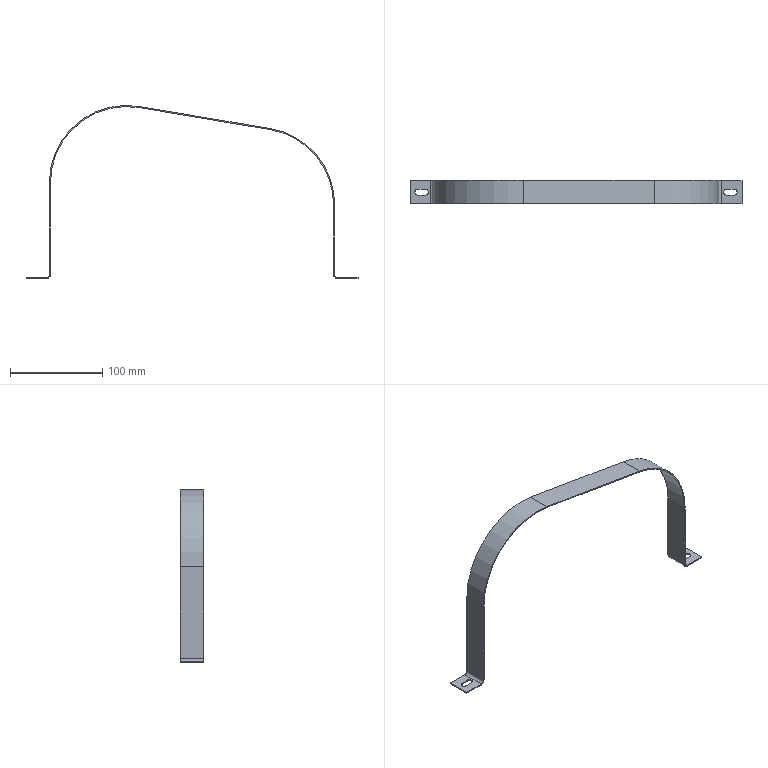Part | STEP file | 冲床-300配套压波_id550_x_t | 1 solid | 30 faces | box 360 x 25 x 187.7 mm | volume 18888 mm3 | plane 18 | cylinder 12 | commonest cylinder face diameters 6.5 x4 6.6 x2 9 x2 165 x2 167.4 x2
STEP:
#1=CARTESIAN_POINT('',(1263.702,135.,185.354));
#2=VERTEX_POINT('',#1);
#3=CARTESIAN_POINT('',(1167.5,135.,104.));
#4=VERTEX_POINT('',#3);
#5=CARTESIAN_POINT('',(1250.,135.,104.));
#6=DIRECTION('',(0.,-1.,0.));
#7=DIRECTION('',(-1.,0.,0.));
#8=AXIS2_PLACEMENT_3D('',#5,#6,#7);
#9=CIRCLE('',#8,82.5);
#10=EDGE_CURVE('',#2,#4,#9,.T.);
#11=ORIENTED_EDGE('',*,*,#10,.T.);
#12=CARTESIAN_POINT('',(1167.5,135.,4.5));
#13=VERTEX_POINT('',#12);
#14=CARTESIAN_POINT('',(1167.5,135.,104.));
#15=DIRECTION('',(0.,0.,-1.));
#16=VECTOR('',#15,1.);
#17=LINE('',#14,#16);
#18=EDGE_CURVE('',#4,#13,#17,.T.);
#19=ORIENTED_EDGE('',*,*,#18,.T.);
#20=CARTESIAN_POINT('',(1163.,135.,0.));
#21=VERTEX_POINT('',#20);
#22=CARTESIAN_POINT('',(1163.,135.,4.5));
#23=DIRECTION('',(0.,1.,0.));
#24=DIRECTION('',(0.,0.,-1.));
#25=AXIS2_PLACEMENT_3D('',#22,#23,#24);
#26=CIRCLE('',#25,4.5);
#27=EDGE_CURVE('',#13,#21,#26,.T.);
#28=ORIENTED_EDGE('',*,*,#27,.T.);
#29=CARTESIAN_POINT('',(1141.,135.,0.));
#30=VERTEX_POINT('',#29);
#31=CARTESIAN_POINT('',(1507.,135.,0.));
#32=DIRECTION('',(1.,0.,0.));
#33=VECTOR('',#32,1.);
#34=LINE('',#31,#33);
#35=EDGE_CURVE('',#30,#21,#34,.T.);
#36=ORIENTED_EDGE('',*,*,#35,.F.);
#37=CARTESIAN_POINT('',(1141.,135.,1.2));
#38=VERTEX_POINT('',#37);
#39=CARTESIAN_POINT('',(1141.,135.,-20.));
#40=DIRECTION('',(0.,0.,1.));
#41=VECTOR('',#40,1.);
#42=LINE('',#39,#41);
#43=EDGE_CURVE('',#30,#38,#42,.T.);
#44=ORIENTED_EDGE('',*,*,#43,.T.);
#45=CARTESIAN_POINT('',(1163.,135.,1.2));
#46=VERTEX_POINT('',#45);
#47=CARTESIAN_POINT('',(1250.,135.,1.2));
#48=DIRECTION('',(1.,0.,0.));
#49=VECTOR('',#48,1.);
#50=LINE('',#47,#49);
#51=EDGE_CURVE('',#38,#46,#50,.T.);
#52=ORIENTED_EDGE('',*,*,#51,.T.);
#53=CARTESIAN_POINT('',(1166.3,135.,4.5));
#54=VERTEX_POINT('',#53);
#55=CARTESIAN_POINT('',(1163.,135.,4.5));
#56=DIRECTION('',(0.,-1.,0.));
#57=DIRECTION('',(-1.,0.,0.));
#58=AXIS2_PLACEMENT_3D('',#55,#56,#57);
#59=CIRCLE('',#58,3.3);
#60=EDGE_CURVE('',#46,#54,#59,.T.);
#61=ORIENTED_EDGE('',*,*,#60,.T.);
#62=CARTESIAN_POINT('',(1166.3,135.,104.));
#63=VERTEX_POINT('',#62);
#64=CARTESIAN_POINT('',(1166.3,135.,104.));
#65=DIRECTION('',(0.,0.,1.));
#66=VECTOR('',#65,1.);
#67=LINE('',#64,#66);
#68=EDGE_CURVE('',#54,#63,#67,.T.);
#69=ORIENTED_EDGE('',*,*,#68,.T.);
#70=CARTESIAN_POINT('',(1263.901,135.,186.537));
#71=VERTEX_POINT('',#70);
#72=CARTESIAN_POINT('',(1250.,135.,104.));
#73=DIRECTION('',(0.,-1.,0.));
#74=DIRECTION('',(-1.,0.,0.));
#75=AXIS2_PLACEMENT_3D('',#72,#73,#74);
#76=CIRCLE('',#75,83.7);
#77=EDGE_CURVE('',#71,#63,#76,.T.);
#78=ORIENTED_EDGE('',*,*,#77,.F.);
#79=CARTESIAN_POINT('',(1405.901,135.,162.621));
#80=VERTEX_POINT('',#79);
#81=CARTESIAN_POINT('',(1405.901,135.,162.621));
#82=DIRECTION('',(-0.9861,0.,0.1661));
#83=VECTOR('',#82,1.);
#84=LINE('',#81,#83);
#85=EDGE_CURVE('',#80,#71,#84,.T.);
#86=ORIENTED_EDGE('',*,*,#85,.F.);
#87=CARTESIAN_POINT('',(1475.7,135.,80.083));
#88=VERTEX_POINT('',#87);
#89=CARTESIAN_POINT('',(1392.,135.,80.083));
#90=DIRECTION('',(0.,-1.,0.));
#91=DIRECTION('',(-1.,0.,0.));
#92=AXIS2_PLACEMENT_3D('',#89,#90,#91);
#93=CIRCLE('',#92,83.7);
#94=EDGE_CURVE('',#88,#80,#93,.T.);
#95=ORIENTED_EDGE('',*,*,#94,.F.);
#96=CARTESIAN_POINT('',(1475.7,135.,4.5));
#97=VERTEX_POINT('',#96);
#98=CARTESIAN_POINT('',(1475.7,135.,0.));
#99=DIRECTION('',(0.,0.,1.));
#100=VECTOR('',#99,1.);
#101=LINE('',#98,#100);
#102=EDGE_CURVE('',#97,#88,#101,.T.);
#103=ORIENTED_EDGE('',*,*,#102,.F.);
#104=CARTESIAN_POINT('',(1479.,135.,1.2));
#105=VERTEX_POINT('',#104);
#106=CARTESIAN_POINT('',(1479.,135.,4.5));
#107=DIRECTION('',(0.,-1.,0.));
#108=DIRECTION('',(-1.,0.,0.));
#109=AXIS2_PLACEMENT_3D('',#106,#107,#108);
#110=CIRCLE('',#109,3.3);
#111=EDGE_CURVE('',#97,#105,#110,.T.);
#112=ORIENTED_EDGE('',*,*,#111,.T.);
#113=CARTESIAN_POINT('',(1501.,135.,1.2));
#114=VERTEX_POINT('',#113);
#115=CARTESIAN_POINT('',(1250.,135.,1.2));
#116=DIRECTION('',(1.,0.,0.));
#117=VECTOR('',#116,1.);
#118=LINE('',#115,#117);
#119=EDGE_CURVE('',#105,#114,#118,.T.);
#120=ORIENTED_EDGE('',*,*,#119,.T.);
#121=CARTESIAN_POINT('',(1501.,135.,0.));
#122=VERTEX_POINT('',#121);
#123=CARTESIAN_POINT('',(1501.,135.,0.));
#124=DIRECTION('',(0.,0.,-1.));
#125=VECTOR('',#124,1.);
#126=LINE('',#123,#125);
#127=EDGE_CURVE('',#114,#122,#126,.T.);
#128=ORIENTED_EDGE('',*,*,#127,.T.);
#129=CARTESIAN_POINT('',(1479.,135.,0.));
#130=VERTEX_POINT('',#129);
#131=CARTESIAN_POINT('',(1507.,135.,0.));
#132=DIRECTION('',(1.,0.,0.));
#133=VECTOR('',#132,1.);
#134=LINE('',#131,#133);
#135=EDGE_CURVE('',#130,#122,#134,.T.);
#136=ORIENTED_EDGE('',*,*,#135,.F.);
#137=CARTESIAN_POINT('',(1474.5,135.,4.5));
#138=VERTEX_POINT('',#137);
#139=CARTESIAN_POINT('',(1479.,135.,4.5));
#140=DIRECTION('',(0.,1.,0.));
#141=DIRECTION('',(0.,0.,-1.));
#142=AXIS2_PLACEMENT_3D('',#139,#140,#141);
#143=CIRCLE('',#142,4.5);
#144=EDGE_CURVE('',#130,#138,#143,.T.);
#145=ORIENTED_EDGE('',*,*,#144,.T.);
#146=CARTESIAN_POINT('',(1474.5,135.,80.083));
#147=VERTEX_POINT('',#146);
#148=CARTESIAN_POINT('',(1474.5,135.,104.));
#149=DIRECTION('',(0.,0.,1.));
#150=VECTOR('',#149,1.);
#151=LINE('',#148,#150);
#152=EDGE_CURVE('',#138,#147,#151,.T.);
#153=ORIENTED_EDGE('',*,*,#152,.T.);
#154=CARTESIAN_POINT('',(1405.702,135.,161.438));
#155=VERTEX_POINT('',#154);
#156=CARTESIAN_POINT('',(1392.,135.,80.083));
#157=DIRECTION('',(0.,-1.,0.));
#158=DIRECTION('',(-1.,0.,0.));
#159=AXIS2_PLACEMENT_3D('',#156,#157,#158);
#160=CIRCLE('',#159,82.5);
#161=EDGE_CURVE('',#147,#155,#160,.T.);
#162=ORIENTED_EDGE('',*,*,#161,.T.);
#163=CARTESIAN_POINT('',(1263.702,135.,185.354));
#164=DIRECTION('',(-0.9861,0.,0.1661));
#165=VECTOR('',#164,1.);
#166=LINE('',#163,#165);
#167=EDGE_CURVE('',#155,#2,#166,.T.);
#168=ORIENTED_EDGE('',*,*,#167,.T.);
#169=EDGE_LOOP('',(#11,#19,#28,#36,#44,#52,#61,#69,#78,#86,#95,#103,#112,#120,#128,#136,#145,#153,#162,#168));
#170=FACE_OUTER_BOUND('',#169,.T.);
#171=CARTESIAN_POINT('',(1250.,135.,104.));
#172=DIRECTION('',(0.,1.,0.));
#173=DIRECTION('',(0.9861,0.,-0.1661));
#174=AXIS2_PLACEMENT_3D('',#171,#172,#173);
#175=PLANE('',#174);
#176=ADVANCED_FACE('',(#170),#175,.T.);
#177=CARTESIAN_POINT('',(1474.5,110.,4.5));
#178=VERTEX_POINT('',#177);
#179=CARTESIAN_POINT('',(1474.5,71.5,4.5));
#180=DIRECTION('',(0.,-1.,0.));
#181=VECTOR('',#180,1.);
#182=LINE('',#179,#181);
#183=EDGE_CURVE('',#138,#178,#182,.T.);
#184=ORIENTED_EDGE('',*,*,#183,.T.);
#185=CARTESIAN_POINT('',(1474.5,110.,80.083));
#186=VERTEX_POINT('',#185);
#187=CARTESIAN_POINT('',(1474.5,110.,0.));
#188=DIRECTION('',(0.,0.,-1.));
#189=VECTOR('',#188,1.);
#190=LINE('',#187,#189);
#191=EDGE_CURVE('',#186,#178,#190,.T.);
#192=ORIENTED_EDGE('',*,*,#191,.F.);
#193=CARTESIAN_POINT('',(1474.5,71.5,80.083));
#194=DIRECTION('',(0.,-1.,0.));
#195=VECTOR('',#194,1.);
#196=LINE('',#193,#195);
#197=EDGE_CURVE('',#147,#186,#196,.T.);
#198=ORIENTED_EDGE('',*,*,#197,.F.);
#199=ORIENTED_EDGE('',*,*,#152,.F.);
#200=EDGE_LOOP('',(#184,#192,#198,#199));
#201=FACE_OUTER_BOUND('',#200,.T.);
#202=CARTESIAN_POINT('',(1474.5,71.5,0.));
#203=DIRECTION('',(1.,0.,0.));
#204=DIRECTION('',(0.,0.,-1.));
#205=AXIS2_PLACEMENT_3D('',#202,#203,#204);
#206=PLANE('',#205);
#207=ADVANCED_FACE('',(#201),#206,.F.);
#208=ORIENTED_EDGE('',*,*,#197,.T.);
#209=CARTESIAN_POINT('',(1405.702,110.,161.438));
#210=VERTEX_POINT('',#209);
#211=CARTESIAN_POINT('',(1392.,110.,80.083));
#212=DIRECTION('',(0.,1.,0.));
#213=DIRECTION('',(0.,0.,1.));
#214=AXIS2_PLACEMENT_3D('',#211,#212,#213);
#215=CIRCLE('',#214,82.5);
#216=EDGE_CURVE('',#210,#186,#215,.T.);
#217=ORIENTED_EDGE('',*,*,#216,.F.);
#218=CARTESIAN_POINT('',(1405.702,71.5,161.438));
#219=DIRECTION('',(0.,-1.,0.));
#220=VECTOR('',#219,1.);
#221=LINE('',#218,#220);
#222=EDGE_CURVE('',#155,#210,#221,.T.);
#223=ORIENTED_EDGE('',*,*,#222,.F.);
#224=ORIENTED_EDGE('',*,*,#161,.F.);
#225=EDGE_LOOP('',(#208,#217,#223,#224));
#226=FACE_OUTER_BOUND('',#225,.T.);
#227=CARTESIAN_POINT('',(1392.,71.5,80.083));
#228=DIRECTION('',(0.,1.,0.));
#229=DIRECTION('',(0.,0.,-1.));
#230=AXIS2_PLACEMENT_3D('',#227,#228,#229);
#231=CYLINDRICAL_SURFACE('',#230,82.5);
#232=ADVANCED_FACE('',(#226),#231,.F.);
#233=ORIENTED_EDGE('',*,*,#51,.F.);
#234=CARTESIAN_POINT('',(1141.,110.,1.2));
#235=VERTEX_POINT('',#234);
#236=CARTESIAN_POINT('',(1141.,-300.,1.2));
#237=DIRECTION('',(0.,1.,0.));
#238=VECTOR('',#237,1.);
#239=LINE('',#236,#238);
#240=EDGE_CURVE('',#235,#38,#239,.T.);
#241=ORIENTED_EDGE('',*,*,#240,.F.);
#242=CARTESIAN_POINT('',(1163.,110.,1.2));
#243=VERTEX_POINT('',#242);
#244=CARTESIAN_POINT('',(1250.,110.,1.2));
#245=DIRECTION('',(-1.,0.,0.));
#246=VECTOR('',#245,1.);
#247=LINE('',#244,#246);
#248=EDGE_CURVE('',#243,#235,#247,.T.);
#249=ORIENTED_EDGE('',*,*,#248,.F.);
#250=CARTESIAN_POINT('',(1163.,71.5,1.2));
#251=DIRECTION('',(0.,-1.,0.));
#252=VECTOR('',#251,1.);
#253=LINE('',#250,#252);
#254=EDGE_CURVE('',#46,#243,#253,.T.);
#255=ORIENTED_EDGE('',*,*,#254,.F.);
#256=EDGE_LOOP('',(#233,#241,#249,#255));
#257=FACE_BOUND('',#256,.T.);
#258=CARTESIAN_POINT('',(1157.5,125.75,1.2));
#259=VERTEX_POINT('',#258);
#260=CARTESIAN_POINT('',(1149.5,125.75,1.2));
#261=VERTEX_POINT('',#260);
#262=CARTESIAN_POINT('',(1157.5,125.75,1.2));
#263=DIRECTION('',(-1.,0.,0.));
#264=VECTOR('',#263,1.);
#265=LINE('',#262,#264);
#266=EDGE_CURVE('',#259,#261,#265,.T.);
#267=ORIENTED_EDGE('',*,*,#266,.F.);
#268=CARTESIAN_POINT('',(1157.5,119.25,1.2));
#269=VERTEX_POINT('',#268);
#270=CARTESIAN_POINT('',(1157.5,122.5,1.2));
#271=DIRECTION('',(0.,0.,1.));
#272=DIRECTION('',(1.,0.,0.));
#273=AXIS2_PLACEMENT_3D('',#270,#271,#272);
#274=CIRCLE('',#273,3.25);
#275=EDGE_CURVE('',#269,#259,#274,.T.);
#276=ORIENTED_EDGE('',*,*,#275,.F.);
#277=CARTESIAN_POINT('',(1149.5,119.25,1.2));
#278=VERTEX_POINT('',#277);
#279=CARTESIAN_POINT('',(1149.5,119.25,1.2));
#280=DIRECTION('',(1.,0.,0.));
#281=VECTOR('',#280,1.);
#282=LINE('',#279,#281);
#283=EDGE_CURVE('',#278,#269,#282,.T.);
#284=ORIENTED_EDGE('',*,*,#283,.F.);
#285=CARTESIAN_POINT('',(1149.5,122.5,1.2));
#286=DIRECTION('',(0.,0.,1.));
#287=DIRECTION('',(1.,0.,0.));
#288=AXIS2_PLACEMENT_3D('',#285,#286,#287);
#289=CIRCLE('',#288,3.25);
#290=EDGE_CURVE('',#261,#278,#289,.T.);
#291=ORIENTED_EDGE('',*,*,#290,.F.);
#292=EDGE_LOOP('',(#267,#276,#284,#291));
#293=FACE_BOUND('',#292,.T.);
#294=CARTESIAN_POINT('',(1165.,71.5,1.2));
#295=DIRECTION('',(0.,0.,1.));
#296=DIRECTION('',(1.,0.,0.));
#297=AXIS2_PLACEMENT_3D('',#294,#295,#296);
#298=PLANE('',#297);
#299=ADVANCED_FACE('',(#257,#293),#298,.T.);
#300=CARTESIAN_POINT('',(1163.,110.,0.));
#301=VERTEX_POINT('',#300);
#302=CARTESIAN_POINT('',(1141.,110.,0.));
#303=VERTEX_POINT('',#302);
#304=CARTESIAN_POINT('',(1507.,110.,0.));
#305=DIRECTION('',(-1.,0.,0.));
#306=VECTOR('',#305,1.);
#307=LINE('',#304,#306);
#308=EDGE_CURVE('',#301,#303,#307,.T.);
#309=ORIENTED_EDGE('',*,*,#308,.T.);
#310=CARTESIAN_POINT('',(1141.,71.5,0.));
#311=DIRECTION('',(0.,1.,0.));
#312=VECTOR('',#311,1.);
#313=LINE('',#310,#312);
#314=EDGE_CURVE('',#303,#30,#313,.T.);
#315=ORIENTED_EDGE('',*,*,#314,.T.);
#316=ORIENTED_EDGE('',*,*,#35,.T.);
#317=CARTESIAN_POINT('',(1163.,71.5,0.));
#318=DIRECTION('',(0.,1.,0.));
#319=VECTOR('',#318,1.);
#320=LINE('',#317,#319);
#321=EDGE_CURVE('',#301,#21,#320,.T.);
#322=ORIENTED_EDGE('',*,*,#321,.F.);
#323=EDGE_LOOP('',(#309,#315,#316,#322));
#324=FACE_BOUND('',#323,.T.);
#325=CARTESIAN_POINT('',(1149.5,125.75,0.));
#326=VERTEX_POINT('',#325);
#327=CARTESIAN_POINT('',(1149.5,119.25,0.));
#328=VERTEX_POINT('',#327);
#329=CARTESIAN_POINT('',(1149.5,122.5,0.));
#330=DIRECTION('',(0.,0.,1.));
#331=DIRECTION('',(1.,0.,0.));
#332=AXIS2_PLACEMENT_3D('',#329,#330,#331);
#333=CIRCLE('',#332,3.25);
#334=EDGE_CURVE('',#326,#328,#333,.T.);
#335=ORIENTED_EDGE('',*,*,#334,.T.);
#336=CARTESIAN_POINT('',(1157.5,119.25,0.));
#337=VERTEX_POINT('',#336);
#338=CARTESIAN_POINT('',(1505.5,119.25,0.));
#339=DIRECTION('',(1.,0.,0.));
#340=VECTOR('',#339,1.);
#341=LINE('',#338,#340);
#342=EDGE_CURVE('',#328,#337,#341,.T.);
#343=ORIENTED_EDGE('',*,*,#342,.T.);
#344=CARTESIAN_POINT('',(1157.5,125.75,0.));
#345=VERTEX_POINT('',#344);
#346=CARTESIAN_POINT('',(1157.5,122.5,0.));
#347=DIRECTION('',(0.,0.,1.));
#348=DIRECTION('',(1.,0.,0.));
#349=AXIS2_PLACEMENT_3D('',#346,#347,#348);
#350=CIRCLE('',#349,3.25);
#351=EDGE_CURVE('',#337,#345,#350,.T.);
#352=ORIENTED_EDGE('',*,*,#351,.T.);
#353=CARTESIAN_POINT('',(1505.5,125.75,0.));
#354=DIRECTION('',(-1.,0.,0.));
#355=VECTOR('',#354,1.);
#356=LINE('',#353,#355);
#357=EDGE_CURVE('',#345,#326,#356,.T.);
#358=ORIENTED_EDGE('',*,*,#357,.T.);
#359=EDGE_LOOP('',(#335,#343,#352,#358));
#360=FACE_BOUND('',#359,.T.);
#361=CARTESIAN_POINT('',(1507.,71.5,0.));
#362=DIRECTION('',(0.,0.,1.));
#363=DIRECTION('',(1.,0.,0.));
#364=AXIS2_PLACEMENT_3D('',#361,#362,#363);
#365=PLANE('',#364);
#366=ADVANCED_FACE('',(#324,#360),#365,.F.);
#367=CARTESIAN_POINT('',(1492.5,125.75,0.));
#368=VERTEX_POINT('',#367);
#369=CARTESIAN_POINT('',(1484.5,125.75,0.));
#370=VERTEX_POINT('',#369);
#371=CARTESIAN_POINT('',(1509.5,125.75,0.));
#372=DIRECTION('',(-1.,0.,0.));
#373=VECTOR('',#372,1.);
#374=LINE('',#371,#373);
#375=EDGE_CURVE('',#368,#370,#374,.T.);
#376=ORIENTED_EDGE('',*,*,#375,.T.);
#377=CARTESIAN_POINT('',(1484.5,119.25,0.));
#378=VERTEX_POINT('',#377);
#379=CARTESIAN_POINT('',(1484.5,122.5,0.));
#380=DIRECTION('',(0.,0.,1.));
#381=DIRECTION('',(1.,0.,0.));
#382=AXIS2_PLACEMENT_3D('',#379,#380,#381);
#383=CIRCLE('',#382,3.25);
#384=EDGE_CURVE('',#370,#378,#383,.T.);
#385=ORIENTED_EDGE('',*,*,#384,.T.);
#386=CARTESIAN_POINT('',(1492.5,119.25,0.));
#387=VERTEX_POINT('',#386);
#388=CARTESIAN_POINT('',(1509.5,119.25,0.));
#389=DIRECTION('',(1.,0.,0.));
#390=VECTOR('',#389,1.);
#391=LINE('',#388,#390);
#392=EDGE_CURVE('',#378,#387,#391,.T.);
#393=ORIENTED_EDGE('',*,*,#392,.T.);
#394=CARTESIAN_POINT('',(1492.5,122.5,0.));
#395=DIRECTION('',(0.,0.,1.));
#396=DIRECTION('',(1.,0.,0.));
#397=AXIS2_PLACEMENT_3D('',#394,#395,#396);
#398=CIRCLE('',#397,3.25);
#399=EDGE_CURVE('',#387,#368,#398,.T.);
#400=ORIENTED_EDGE('',*,*,#399,.T.);
#401=EDGE_LOOP('',(#376,#385,#393,#400));
#402=FACE_BOUND('',#401,.T.);
#403=ORIENTED_EDGE('',*,*,#135,.T.);
#404=CARTESIAN_POINT('',(1501.,110.,0.));
#405=VERTEX_POINT('',#404);
#406=CARTESIAN_POINT('',(1501.,71.5,0.));
#407=DIRECTION('',(0.,1.,0.));
#408=VECTOR('',#407,1.);
#409=LINE('',#406,#408);
#410=EDGE_CURVE('',#405,#122,#409,.T.);
#411=ORIENTED_EDGE('',*,*,#410,.F.);
#412=CARTESIAN_POINT('',(1479.,110.,0.));
#413=VERTEX_POINT('',#412);
#414=CARTESIAN_POINT('',(1507.,110.,0.));
#415=DIRECTION('',(-1.,0.,0.));
#416=VECTOR('',#415,1.);
#417=LINE('',#414,#416);
#418=EDGE_CURVE('',#405,#413,#417,.T.);
#419=ORIENTED_EDGE('',*,*,#418,.T.);
#420=CARTESIAN_POINT('',(1479.,71.5,0.));
#421=DIRECTION('',(0.,-1.,0.));
#422=VECTOR('',#421,1.);
#423=LINE('',#420,#422);
#424=EDGE_CURVE('',#130,#413,#423,.T.);
#425=ORIENTED_EDGE('',*,*,#424,.F.);
#426=EDGE_LOOP('',(#403,#411,#419,#425));
#427=FACE_BOUND('',#426,.T.);
#428=CARTESIAN_POINT('',(1507.,71.5,0.));
#429=DIRECTION('',(0.,0.,1.));
#430=DIRECTION('',(1.,0.,0.));
#431=AXIS2_PLACEMENT_3D('',#428,#429,#430);
#432=PLANE('',#431);
#433=ADVANCED_FACE('',(#402,#427),#432,.F.);
#434=CARTESIAN_POINT('',(1475.7,110.,80.083));
#435=VERTEX_POINT('',#434);
#436=CARTESIAN_POINT('',(1475.7,71.5,80.083));
#437=DIRECTION('',(0.,-1.,0.));
#438=VECTOR('',#437,1.);
#439=LINE('',#436,#438);
#440=EDGE_CURVE('',#88,#435,#439,.T.);
#441=ORIENTED_EDGE('',*,*,#440,.F.);
#442=ORIENTED_EDGE('',*,*,#94,.T.);
#443=CARTESIAN_POINT('',(1405.901,110.,162.621));
#444=VERTEX_POINT('',#443);
#445=CARTESIAN_POINT('',(1405.901,71.5,162.621));
#446=DIRECTION('',(0.,-1.,0.));
#447=VECTOR('',#446,1.);
#448=LINE('',#445,#447);
#449=EDGE_CURVE('',#80,#444,#448,.T.);
#450=ORIENTED_EDGE('',*,*,#449,.T.);
#451=CARTESIAN_POINT('',(1392.,110.,80.083));
#452=DIRECTION('',(0.,-1.,0.));
#453=DIRECTION('',(1.,0.,0.));
#454=AXIS2_PLACEMENT_3D('',#451,#452,#453);
#455=CIRCLE('',#454,83.7);
#456=EDGE_CURVE('',#435,#444,#455,.T.);
#457=ORIENTED_EDGE('',*,*,#456,.F.);
#458=EDGE_LOOP('',(#441,#442,#450,#457));
#459=FACE_OUTER_BOUND('',#458,.T.);
#460=CARTESIAN_POINT('',(1392.,71.5,80.083));
#461=DIRECTION('',(0.,1.,0.));
#462=DIRECTION('',(0.,0.,-1.));
#463=AXIS2_PLACEMENT_3D('',#460,#461,#462);
#464=CYLINDRICAL_SURFACE('',#463,83.7);
#465=ADVANCED_FACE('',(#459),#464,.T.);
#466=CARTESIAN_POINT('',(1263.901,110.,186.537));
#467=VERTEX_POINT('',#466);
#468=CARTESIAN_POINT('',(1263.901,71.5,186.537));
#469=DIRECTION('',(0.,-1.,0.));
#470=VECTOR('',#469,1.);
#471=LINE('',#468,#470);
#472=EDGE_CURVE('',#71,#467,#471,.T.);
#473=ORIENTED_EDGE('',*,*,#472,.F.);
#474=ORIENTED_EDGE('',*,*,#77,.T.);
#475=CARTESIAN_POINT('',(1166.3,110.,104.));
#476=VERTEX_POINT('',#475);
#477=CARTESIAN_POINT('',(1166.3,71.5,104.));
#478=DIRECTION('',(0.,-1.,0.));
#479=VECTOR('',#478,1.);
#480=LINE('',#477,#479);
#481=EDGE_CURVE('',#63,#476,#480,.T.);
#482=ORIENTED_EDGE('',*,*,#481,.T.);
#483=CARTESIAN_POINT('',(1250.,110.,104.));
#484=DIRECTION('',(0.,-1.,0.));
#485=DIRECTION('',(1.,0.,0.));
#486=AXIS2_PLACEMENT_3D('',#483,#484,#485);
#487=CIRCLE('',#486,83.7);
#488=EDGE_CURVE('',#467,#476,#487,.T.);
#489=ORIENTED_EDGE('',*,*,#488,.F.);
#490=EDGE_LOOP('',(#473,#474,#482,#489));
#491=FACE_OUTER_BOUND('',#490,.T.);
#492=CARTESIAN_POINT('',(1250.,71.5,104.));
#493=DIRECTION('',(0.,1.,0.));
#494=DIRECTION('',(0.,0.,-1.));
#495=AXIS2_PLACEMENT_3D('',#492,#493,#494);
#496=CYLINDRICAL_SURFACE('',#495,83.7);
#497=ADVANCED_FACE('',(#491),#496,.T.);
#498=ORIENTED_EDGE('',*,*,#240,.T.);
#499=ORIENTED_EDGE('',*,*,#43,.F.);
#500=ORIENTED_EDGE('',*,*,#314,.F.);
#501=CARTESIAN_POINT('',(1141.,110.,-20.));
#502=DIRECTION('',(0.,0.,-1.));
#503=VECTOR('',#502,1.);
#504=LINE('',#501,#503);
#505=EDGE_CURVE('',#235,#303,#504,.T.);
#506=ORIENTED_EDGE('',*,*,#505,.F.);
#507=EDGE_LOOP('',(#498,#499,#500,#506));
#508=FACE_OUTER_BOUND('',#507,.T.);
#509=CARTESIAN_POINT('',(1141.,-300.,-20.));
#510=DIRECTION('',(-1.,0.,0.));
#511=DIRECTION('',(0.,0.,1.));
#512=AXIS2_PLACEMENT_3D('',#509,#510,#511);
#513=PLANE('',#512);
#514=ADVANCED_FACE('',(#508),#513,.T.);
#515=ORIENTED_EDGE('',*,*,#410,.T.);
#516=ORIENTED_EDGE('',*,*,#127,.F.);
#517=CARTESIAN_POINT('',(1501.,110.,1.2));
#518=VERTEX_POINT('',#517);
#519=CARTESIAN_POINT('',(1501.,71.5,1.2));
#520=DIRECTION('',(0.,1.,0.));
#521=VECTOR('',#520,1.);
#522=LINE('',#519,#521);
#523=EDGE_CURVE('',#518,#114,#522,.T.);
#524=ORIENTED_EDGE('',*,*,#523,.F.);
#525=CARTESIAN_POINT('',(1501.,110.,0.));
#526=DIRECTION('',(0.,0.,1.));
#527=VECTOR('',#526,1.);
#528=LINE('',#525,#527);
#529=EDGE_CURVE('',#405,#518,#528,.T.);
#530=ORIENTED_EDGE('',*,*,#529,.F.);
#531=EDGE_LOOP('',(#515,#516,#524,#530));
#532=FACE_OUTER_BOUND('',#531,.T.);
#533=CARTESIAN_POINT('',(1501.,71.5,0.));
#534=DIRECTION('',(-1.,0.,0.));
#535=DIRECTION('',(0.,1.,0.));
#536=AXIS2_PLACEMENT_3D('',#533,#534,#535);
#537=PLANE('',#536);
#538=ADVANCED_FACE('',(#532),#537,.F.);
#539=CARTESIAN_POINT('',(1492.5,119.25,1.2));
#540=VERTEX_POINT('',#539);
#541=CARTESIAN_POINT('',(1492.5,125.75,1.2));
#542=VERTEX_POINT('',#541);
#543=CARTESIAN_POINT('',(1492.5,122.5,1.2));
#544=DIRECTION('',(0.,0.,1.));
#545=DIRECTION('',(1.,0.,0.));
#546=AXIS2_PLACEMENT_3D('',#543,#544,#545);
#547=CIRCLE('',#546,3.25);
#548=EDGE_CURVE('',#540,#542,#547,.T.);
#549=ORIENTED_EDGE('',*,*,#548,.F.);
#550=CARTESIAN_POINT('',(1484.5,119.25,1.2));
#551=VERTEX_POINT('',#550);
#552=CARTESIAN_POINT('',(1484.5,119.25,1.2));
#553=DIRECTION('',(1.,0.,0.));
#554=VECTOR('',#553,1.);
#555=LINE('',#552,#554);
#556=EDGE_CURVE('',#551,#540,#555,.T.);
#557=ORIENTED_EDGE('',*,*,#556,.F.);
#558=CARTESIAN_POINT('',(1484.5,125.75,1.2));
#559=VERTEX_POINT('',#558);
#560=CARTESIAN_POINT('',(1484.5,122.5,1.2));
#561=DIRECTION('',(0.,0.,1.));
#562=DIRECTION('',(1.,0.,0.));
#563=AXIS2_PLACEMENT_3D('',#560,#561,#562);
#564=CIRCLE('',#563,3.25);
#565=EDGE_CURVE('',#559,#551,#564,.T.);
#566=ORIENTED_EDGE('',*,*,#565,.F.);
#567=CARTESIAN_POINT('',(1492.5,125.75,1.2));
#568=DIRECTION('',(-1.,0.,0.));
#569=VECTOR('',#568,1.);
#570=LINE('',#567,#569);
#571=EDGE_CURVE('',#542,#559,#570,.T.);
#572=ORIENTED_EDGE('',*,*,#571,.F.);
#573=EDGE_LOOP('',(#549,#557,#566,#572));
#574=FACE_BOUND('',#573,.T.);
#575=CARTESIAN_POINT('',(1479.,110.,1.2));
#576=VERTEX_POINT('',#575);
#577=CARTESIAN_POINT('',(1250.,110.,1.2));
#578=DIRECTION('',(-1.,0.,0.));
#579=VECTOR('',#578,1.);
#580=LINE('',#577,#579);
#581=EDGE_CURVE('',#518,#576,#580,.T.);
#582=ORIENTED_EDGE('',*,*,#581,.F.);
#583=ORIENTED_EDGE('',*,*,#523,.T.);
#584=ORIENTED_EDGE('',*,*,#119,.F.);
#585=CARTESIAN_POINT('',(1479.,71.5,1.2));
#586=DIRECTION('',(0.,1.,0.));
#587=VECTOR('',#586,1.);
#588=LINE('',#585,#587);
#589=EDGE_CURVE('',#576,#105,#588,.T.);
#590=ORIENTED_EDGE('',*,*,#589,.F.);
#591=EDGE_LOOP('',(#582,#583,#584,#590));
#592=FACE_BOUND('',#591,.T.);
#593=CARTESIAN_POINT('',(1507.,71.5,1.2));
#594=DIRECTION('',(0.,0.,1.));
#595=DIRECTION('',(1.,0.,0.));
#596=AXIS2_PLACEMENT_3D('',#593,#594,#595);
#597=PLANE('',#596);
#598=ADVANCED_FACE('',(#574,#592),#597,.T.);
#599=ORIENTED_EDGE('',*,*,#102,.T.);
#600=ORIENTED_EDGE('',*,*,#440,.T.);
#601=CARTESIAN_POINT('',(1475.7,110.,4.5));
#602=VERTEX_POINT('',#601);
#603=CARTESIAN_POINT('',(1475.7,110.,104.));
#604=DIRECTION('',(0.,0.,1.));
#605=VECTOR('',#604,1.);
#606=LINE('',#603,#605);
#607=EDGE_CURVE('',#602,#435,#606,.T.);
#608=ORIENTED_EDGE('',*,*,#607,.F.);
#609=CARTESIAN_POINT('',(1475.7,71.5,4.5));
#610=DIRECTION('',(0.,-1.,0.));
#611=VECTOR('',#610,1.);
#612=LINE('',#609,#611);
#613=EDGE_CURVE('',#97,#602,#612,.T.);
#614=ORIENTED_EDGE('',*,*,#613,.F.);
#615=EDGE_LOOP('',(#599,#600,#608,#614));
#616=FACE_OUTER_BOUND('',#615,.T.);
#617=CARTESIAN_POINT('',(1475.7,71.5,0.));
#618=DIRECTION('',(1.,0.,0.));
#619=DIRECTION('',(0.,0.,-1.));
#620=AXIS2_PLACEMENT_3D('',#617,#618,#619);
#621=PLANE('',#620);
#622=ADVANCED_FACE('',(#616),#621,.T.);
#623=ORIENTED_EDGE('',*,*,#449,.F.);
#624=ORIENTED_EDGE('',*,*,#85,.T.);
#625=ORIENTED_EDGE('',*,*,#472,.T.);
#626=CARTESIAN_POINT('',(1263.901,110.,186.537));
#627=DIRECTION('',(-0.9861,0.,0.1661));
#628=VECTOR('',#627,1.);
#629=LINE('',#626,#628);
#630=EDGE_CURVE('',#444,#467,#629,.T.);
#631=ORIENTED_EDGE('',*,*,#630,.F.);
#632=EDGE_LOOP('',(#623,#624,#625,#631));
#633=FACE_OUTER_BOUND('',#632,.T.);
#634=CARTESIAN_POINT('',(1405.901,71.5,162.621));
#635=DIRECTION('',(0.1661,0.,0.9861));
#636=DIRECTION('',(0.9861,0.,-0.1661));
#637=AXIS2_PLACEMENT_3D('',#634,#635,#636);
#638=PLANE('',#637);
#639=ADVANCED_FACE('',(#633),#638,.T.);
#640=CARTESIAN_POINT('',(1166.3,110.,4.5));
#641=VERTEX_POINT('',#640);
#642=CARTESIAN_POINT('',(1166.3,110.,104.));
#643=DIRECTION('',(0.,0.,-1.));
#644=VECTOR('',#643,1.);
#645=LINE('',#642,#644);
#646=EDGE_CURVE('',#476,#641,#645,.T.);
#647=ORIENTED_EDGE('',*,*,#646,.F.);
#648=ORIENTED_EDGE('',*,*,#481,.F.);
#649=ORIENTED_EDGE('',*,*,#68,.F.);
#650=CARTESIAN_POINT('',(1166.3,71.5,4.5));
#651=DIRECTION('',(0.,1.,0.));
#652=VECTOR('',#651,1.);
#653=LINE('',#650,#652);
#654=EDGE_CURVE('',#641,#54,#653,.T.);
#655=ORIENTED_EDGE('',*,*,#654,.F.);
#656=EDGE_LOOP('',(#647,#648,#649,#655));
#657=FACE_OUTER_BOUND('',#656,.T.);
#658=CARTESIAN_POINT('',(1166.3,71.5,104.));
#659=DIRECTION('',(-1.,0.,0.));
#660=DIRECTION('',(0.,0.,1.));
#661=AXIS2_PLACEMENT_3D('',#658,#659,#660);
#662=PLANE('',#661);
#663=ADVANCED_FACE('',(#657),#662,.T.);
#664=CARTESIAN_POINT('',(1167.5,110.,4.5));
#665=VERTEX_POINT('',#664);
#666=CARTESIAN_POINT('',(1167.5,110.,104.));
#667=VERTEX_POINT('',#666);
#668=CARTESIAN_POINT('',(1167.5,110.,104.));
#669=DIRECTION('',(0.,0.,1.));
#670=VECTOR('',#669,1.);
#671=LINE('',#668,#670);
#672=EDGE_CURVE('',#665,#667,#671,.T.);
#673=ORIENTED_EDGE('',*,*,#672,.T.);
#674=CARTESIAN_POINT('',(1263.702,110.,185.354));
#675=VERTEX_POINT('',#674);
#676=CARTESIAN_POINT('',(1250.,110.,104.));
#677=DIRECTION('',(0.,1.,0.));
#678=DIRECTION('',(0.,0.,1.));
#679=AXIS2_PLACEMENT_3D('',#676,#677,#678);
#680=CIRCLE('',#679,82.5);
#681=EDGE_CURVE('',#667,#675,#680,.T.);
#682=ORIENTED_EDGE('',*,*,#681,.T.);
#683=CARTESIAN_POINT('',(1405.702,110.,161.438));
#684=DIRECTION('',(0.9861,0.,-0.1661));
#685=VECTOR('',#684,1.);
#686=LINE('',#683,#685);
#687=EDGE_CURVE('',#675,#210,#686,.T.);
#688=ORIENTED_EDGE('',*,*,#687,.T.);
#689=ORIENTED_EDGE('',*,*,#216,.T.);
#690=ORIENTED_EDGE('',*,*,#191,.T.);
#691=CARTESIAN_POINT('',(1479.,110.,4.5));
#692=DIRECTION('',(0.,-1.,0.));
#693=DIRECTION('',(0.,0.,1.));
#694=AXIS2_PLACEMENT_3D('',#691,#692,#693);
#695=CIRCLE('',#694,4.5);
#696=EDGE_CURVE('',#178,#413,#695,.T.);
#697=ORIENTED_EDGE('',*,*,#696,.T.);
#698=ORIENTED_EDGE('',*,*,#418,.F.);
#699=ORIENTED_EDGE('',*,*,#529,.T.);
#700=ORIENTED_EDGE('',*,*,#581,.T.);
#701=CARTESIAN_POINT('',(1479.,110.,4.5));
#702=DIRECTION('',(0.,1.,0.));
#703=DIRECTION('',(1.,0.,0.));
#704=AXIS2_PLACEMENT_3D('',#701,#702,#703);
#705=CIRCLE('',#704,3.3);
#706=EDGE_CURVE('',#576,#602,#705,.T.);
#707=ORIENTED_EDGE('',*,*,#706,.T.);
#708=ORIENTED_EDGE('',*,*,#607,.T.);
#709=ORIENTED_EDGE('',*,*,#456,.T.);
#710=ORIENTED_EDGE('',*,*,#630,.T.);
#711=ORIENTED_EDGE('',*,*,#488,.T.);
#712=ORIENTED_EDGE('',*,*,#646,.T.);
#713=CARTESIAN_POINT('',(1163.,110.,4.5));
#714=DIRECTION('',(0.,1.,0.));
#715=DIRECTION('',(1.,0.,0.));
#716=AXIS2_PLACEMENT_3D('',#713,#714,#715);
#717=CIRCLE('',#716,3.3);
#718=EDGE_CURVE('',#641,#243,#717,.T.);
#719=ORIENTED_EDGE('',*,*,#718,.T.);
#720=ORIENTED_EDGE('',*,*,#248,.T.);
#721=ORIENTED_EDGE('',*,*,#505,.T.);
#722=ORIENTED_EDGE('',*,*,#308,.F.);
#723=CARTESIAN_POINT('',(1163.,110.,4.5));
#724=DIRECTION('',(0.,-1.,0.));
#725=DIRECTION('',(0.,0.,1.));
#726=AXIS2_PLACEMENT_3D('',#723,#724,#725);
#727=CIRCLE('',#726,4.5);
#728=EDGE_CURVE('',#301,#665,#727,.T.);
#729=ORIENTED_EDGE('',*,*,#728,.T.);
#730=EDGE_LOOP('',(#673,#682,#688,#689,#690,#697,#698,#699,#700,#707,#708,#709,#710,#711,#712,#719,#720,#721,#722,#729));
#731=FACE_OUTER_BOUND('',#730,.T.);
#732=CARTESIAN_POINT('',(1250.,110.,104.));
#733=DIRECTION('',(0.,-1.,0.));
#734=DIRECTION('',(-0.9861,0.,0.1661));
#735=AXIS2_PLACEMENT_3D('',#732,#733,#734);
#736=PLANE('',#735);
#737=ADVANCED_FACE('',(#731),#736,.T.);
#738=CARTESIAN_POINT('',(1167.5,71.5,4.5));
#739=DIRECTION('',(0.,1.,0.));
#740=VECTOR('',#739,1.);
#741=LINE('',#738,#740);
#742=EDGE_CURVE('',#665,#13,#741,.T.);
#743=ORIENTED_EDGE('',*,*,#742,.T.);
#744=ORIENTED_EDGE('',*,*,#18,.F.);
#745=CARTESIAN_POINT('',(1167.5,71.5,104.));
#746=DIRECTION('',(0.,-1.,0.));
#747=VECTOR('',#746,1.);
#748=LINE('',#745,#747);
#749=EDGE_CURVE('',#4,#667,#748,.T.);
#750=ORIENTED_EDGE('',*,*,#749,.T.);
#751=ORIENTED_EDGE('',*,*,#672,.F.);
#752=EDGE_LOOP('',(#743,#744,#750,#751));
#753=FACE_OUTER_BOUND('',#752,.T.);
#754=CARTESIAN_POINT('',(1167.5,71.5,104.));
#755=DIRECTION('',(-1.,0.,0.));
#756=DIRECTION('',(0.,0.,1.));
#757=AXIS2_PLACEMENT_3D('',#754,#755,#756);
#758=PLANE('',#757);
#759=ADVANCED_FACE('',(#753),#758,.F.);
#760=ORIENTED_EDGE('',*,*,#749,.F.);
#761=ORIENTED_EDGE('',*,*,#10,.F.);
#762=CARTESIAN_POINT('',(1263.702,71.5,185.354));
#763=DIRECTION('',(0.,-1.,0.));
#764=VECTOR('',#763,1.);
#765=LINE('',#762,#764);
#766=EDGE_CURVE('',#2,#675,#765,.T.);
#767=ORIENTED_EDGE('',*,*,#766,.T.);
#768=ORIENTED_EDGE('',*,*,#681,.F.);
#769=EDGE_LOOP('',(#760,#761,#767,#768));
#770=FACE_OUTER_BOUND('',#769,.T.);
#771=CARTESIAN_POINT('',(1250.,71.5,104.));
#772=DIRECTION('',(0.,1.,0.));
#773=DIRECTION('',(0.,0.,-1.));
#774=AXIS2_PLACEMENT_3D('',#771,#772,#773);
#775=CYLINDRICAL_SURFACE('',#774,82.5);
#776=ADVANCED_FACE('',(#770),#775,.F.);
#777=ORIENTED_EDGE('',*,*,#766,.F.);
#778=ORIENTED_EDGE('',*,*,#167,.F.);
#779=ORIENTED_EDGE('',*,*,#222,.T.);
#780=ORIENTED_EDGE('',*,*,#687,.F.);
#781=EDGE_LOOP('',(#777,#778,#779,#780));
#782=FACE_OUTER_BOUND('',#781,.T.);
#783=CARTESIAN_POINT('',(1405.702,71.5,161.438));
#784=DIRECTION('',(0.1661,0.,0.9861));
#785=DIRECTION('',(0.9861,0.,-0.1661));
#786=AXIS2_PLACEMENT_3D('',#783,#784,#785);
#787=PLANE('',#786);
#788=ADVANCED_FACE('',(#782),#787,.F.);
#789=CARTESIAN_POINT('',(1149.5,125.75,-118.5));
#790=DIRECTION('',(0.,0.,1.));
#791=VECTOR('',#790,1.);
#792=LINE('',#789,#791);
#793=EDGE_CURVE('',#326,#261,#792,.T.);
#794=ORIENTED_EDGE('',*,*,#793,.T.);
#795=ORIENTED_EDGE('',*,*,#290,.T.);
#796=CARTESIAN_POINT('',(1149.5,119.25,-118.5));
#797=DIRECTION('',(0.,0.,1.));
#798=VECTOR('',#797,1.);
#799=LINE('',#796,#798);
#800=EDGE_CURVE('',#328,#278,#799,.T.);
#801=ORIENTED_EDGE('',*,*,#800,.F.);
#802=ORIENTED_EDGE('',*,*,#334,.F.);
#803=EDGE_LOOP('',(#794,#795,#801,#802));
#804=FACE_OUTER_BOUND('',#803,.T.);
#805=CARTESIAN_POINT('',(1149.5,122.5,-118.5));
#806=DIRECTION('',(0.,0.,1.));
#807=DIRECTION('',(1.,0.,0.));
#808=AXIS2_PLACEMENT_3D('',#805,#806,#807);
#809=CYLINDRICAL_SURFACE('',#808,3.25);
#810=ADVANCED_FACE('',(#804),#809,.F.);
#811=ORIENTED_EDGE('',*,*,#800,.T.);
#812=ORIENTED_EDGE('',*,*,#283,.T.);
#813=CARTESIAN_POINT('',(1157.5,119.25,-118.5));
#814=DIRECTION('',(0.,0.,1.));
#815=VECTOR('',#814,1.);
#816=LINE('',#813,#815);
#817=EDGE_CURVE('',#337,#269,#816,.T.);
#818=ORIENTED_EDGE('',*,*,#817,.F.);
#819=ORIENTED_EDGE('',*,*,#342,.F.);
#820=EDGE_LOOP('',(#811,#812,#818,#819));
#821=FACE_OUTER_BOUND('',#820,.T.);
#822=CARTESIAN_POINT('',(1149.5,119.25,-118.5));
#823=DIRECTION('',(0.,1.,0.));
#824=DIRECTION('',(0.,0.,-1.));
#825=AXIS2_PLACEMENT_3D('',#822,#823,#824);
#826=PLANE('',#825);
#827=ADVANCED_FACE('',(#821),#826,.T.);
#828=ORIENTED_EDGE('',*,*,#817,.T.);
#829=ORIENTED_EDGE('',*,*,#275,.T.);
#830=CARTESIAN_POINT('',(1157.5,125.75,-118.5));
#831=DIRECTION('',(0.,0.,1.));
#832=VECTOR('',#831,1.);
#833=LINE('',#830,#832);
#834=EDGE_CURVE('',#345,#259,#833,.T.);
#835=ORIENTED_EDGE('',*,*,#834,.F.);
#836=ORIENTED_EDGE('',*,*,#351,.F.);
#837=EDGE_LOOP('',(#828,#829,#835,#836));
#838=FACE_OUTER_BOUND('',#837,.T.);
#839=CARTESIAN_POINT('',(1157.5,122.5,-118.5));
#840=DIRECTION('',(0.,0.,1.));
#841=DIRECTION('',(1.,0.,0.));
#842=AXIS2_PLACEMENT_3D('',#839,#840,#841);
#843=CYLINDRICAL_SURFACE('',#842,3.25);
#844=ADVANCED_FACE('',(#838),#843,.F.);
#845=ORIENTED_EDGE('',*,*,#834,.T.);
#846=ORIENTED_EDGE('',*,*,#266,.T.);
#847=ORIENTED_EDGE('',*,*,#793,.F.);
#848=ORIENTED_EDGE('',*,*,#357,.F.);
#849=EDGE_LOOP('',(#845,#846,#847,#848));
#850=FACE_OUTER_BOUND('',#849,.T.);
#851=CARTESIAN_POINT('',(1157.5,125.75,-118.5));
#852=DIRECTION('',(0.,-1.,0.));
#853=DIRECTION('',(0.,0.,1.));
#854=AXIS2_PLACEMENT_3D('',#851,#852,#853);
#855=PLANE('',#854);
#856=ADVANCED_FACE('',(#850),#855,.T.);
#857=ORIENTED_EDGE('',*,*,#375,.F.);
#858=CARTESIAN_POINT('',(1492.5,125.75,-118.5));
#859=DIRECTION('',(0.,0.,1.));
#860=VECTOR('',#859,1.);
#861=LINE('',#858,#860);
#862=EDGE_CURVE('',#368,#542,#861,.T.);
#863=ORIENTED_EDGE('',*,*,#862,.T.);
#864=ORIENTED_EDGE('',*,*,#571,.T.);
#865=CARTESIAN_POINT('',(1484.5,125.75,-118.5));
#866=DIRECTION('',(0.,0.,1.));
#867=VECTOR('',#866,1.);
#868=LINE('',#865,#867);
#869=EDGE_CURVE('',#370,#559,#868,.T.);
#870=ORIENTED_EDGE('',*,*,#869,.F.);
#871=EDGE_LOOP('',(#857,#863,#864,#870));
#872=FACE_OUTER_BOUND('',#871,.T.);
#873=CARTESIAN_POINT('',(1492.5,125.75,-118.5));
#874=DIRECTION('',(0.,-1.,0.));
#875=DIRECTION('',(0.,0.,1.));
#876=AXIS2_PLACEMENT_3D('',#873,#874,#875);
#877=PLANE('',#876);
#878=ADVANCED_FACE('',(#872),#877,.T.);
#879=ORIENTED_EDGE('',*,*,#384,.F.);
#880=ORIENTED_EDGE('',*,*,#869,.T.);
#881=ORIENTED_EDGE('',*,*,#565,.T.);
#882=CARTESIAN_POINT('',(1484.5,119.25,-118.5));
#883=DIRECTION('',(0.,0.,1.));
#884=VECTOR('',#883,1.);
#885=LINE('',#882,#884);
#886=EDGE_CURVE('',#378,#551,#885,.T.);
#887=ORIENTED_EDGE('',*,*,#886,.F.);
#888=EDGE_LOOP('',(#879,#880,#881,#887));
#889=FACE_OUTER_BOUND('',#888,.T.);
#890=CARTESIAN_POINT('',(1484.5,122.5,-118.5));
#891=DIRECTION('',(0.,0.,1.));
#892=DIRECTION('',(1.,0.,0.));
#893=AXIS2_PLACEMENT_3D('',#890,#891,#892);
#894=CYLINDRICAL_SURFACE('',#893,3.25);
#895=ADVANCED_FACE('',(#889),#894,.F.);
#896=ORIENTED_EDGE('',*,*,#392,.F.);
#897=ORIENTED_EDGE('',*,*,#886,.T.);
#898=ORIENTED_EDGE('',*,*,#556,.T.);
#899=CARTESIAN_POINT('',(1492.5,119.25,-118.5));
#900=DIRECTION('',(0.,0.,1.));
#901=VECTOR('',#900,1.);
#902=LINE('',#899,#901);
#903=EDGE_CURVE('',#387,#540,#902,.T.);
#904=ORIENTED_EDGE('',*,*,#903,.F.);
#905=EDGE_LOOP('',(#896,#897,#898,#904));
#906=FACE_OUTER_BOUND('',#905,.T.);
#907=CARTESIAN_POINT('',(1484.5,119.25,-118.5));
#908=DIRECTION('',(0.,1.,0.));
#909=DIRECTION('',(0.,0.,-1.));
#910=AXIS2_PLACEMENT_3D('',#907,#908,#909);
#911=PLANE('',#910);
#912=ADVANCED_FACE('',(#906),#911,.T.);
#913=ORIENTED_EDGE('',*,*,#399,.F.);
#914=ORIENTED_EDGE('',*,*,#903,.T.);
#915=ORIENTED_EDGE('',*,*,#548,.T.);
#916=ORIENTED_EDGE('',*,*,#862,.F.);
#917=EDGE_LOOP('',(#913,#914,#915,#916));
#918=FACE_OUTER_BOUND('',#917,.T.);
#919=CARTESIAN_POINT('',(1492.5,122.5,-118.5));
#920=DIRECTION('',(0.,0.,1.));
#921=DIRECTION('',(1.,0.,0.));
#922=AXIS2_PLACEMENT_3D('',#919,#920,#921);
#923=CYLINDRICAL_SURFACE('',#922,3.25);
#924=ADVANCED_FACE('',(#918),#923,.F.);
#925=ORIENTED_EDGE('',*,*,#706,.F.);
#926=ORIENTED_EDGE('',*,*,#589,.T.);
#927=ORIENTED_EDGE('',*,*,#111,.F.);
#928=ORIENTED_EDGE('',*,*,#613,.T.);
#929=EDGE_LOOP('',(#925,#926,#927,#928));
#930=FACE_OUTER_BOUND('',#929,.T.);
#931=CARTESIAN_POINT('',(1479.,71.5,4.5));
#932=DIRECTION('',(0.,-1.,0.));
#933=DIRECTION('',(0.,0.,1.));
#934=AXIS2_PLACEMENT_3D('',#931,#932,#933);
#935=CYLINDRICAL_SURFACE('',#934,3.3);
#936=ADVANCED_FACE('',(#930),#935,.F.);
#937=ORIENTED_EDGE('',*,*,#144,.F.);
#938=ORIENTED_EDGE('',*,*,#424,.T.);
#939=ORIENTED_EDGE('',*,*,#696,.F.);
#940=ORIENTED_EDGE('',*,*,#183,.F.);
#941=EDGE_LOOP('',(#937,#938,#939,#940));
#942=FACE_OUTER_BOUND('',#941,.T.);
#943=CARTESIAN_POINT('',(1479.,71.5,4.5));
#944=DIRECTION('',(0.,-1.,0.));
#945=DIRECTION('',(0.,0.,1.));
#946=AXIS2_PLACEMENT_3D('',#943,#944,#945);
#947=CYLINDRICAL_SURFACE('',#946,4.5);
#948=ADVANCED_FACE('',(#942),#947,.T.);
#949=ORIENTED_EDGE('',*,*,#718,.F.);
#950=ORIENTED_EDGE('',*,*,#654,.T.);
#951=ORIENTED_EDGE('',*,*,#60,.F.);
#952=ORIENTED_EDGE('',*,*,#254,.T.);
#953=EDGE_LOOP('',(#949,#950,#951,#952));
#954=FACE_OUTER_BOUND('',#953,.T.);
#955=CARTESIAN_POINT('',(1163.,71.5,4.5));
#956=DIRECTION('',(0.,-1.,0.));
#957=DIRECTION('',(0.,0.,1.));
#958=AXIS2_PLACEMENT_3D('',#955,#956,#957);
#959=CYLINDRICAL_SURFACE('',#958,3.3);
#960=ADVANCED_FACE('',(#954),#959,.F.);
#961=ORIENTED_EDGE('',*,*,#27,.F.);
#962=ORIENTED_EDGE('',*,*,#742,.F.);
#963=ORIENTED_EDGE('',*,*,#728,.F.);
#964=ORIENTED_EDGE('',*,*,#321,.T.);
#965=EDGE_LOOP('',(#961,#962,#963,#964));
#966=FACE_OUTER_BOUND('',#965,.T.);
#967=CARTESIAN_POINT('',(1163.,71.5,4.5));
#968=DIRECTION('',(0.,-1.,0.));
#969=DIRECTION('',(0.,0.,1.));
#970=AXIS2_PLACEMENT_3D('',#967,#968,#969);
#971=CYLINDRICAL_SURFACE('',#970,4.5);
#972=ADVANCED_FACE('',(#966),#971,.T.);
#973=CLOSED_SHELL('',(#176,#207,#232,#299,#366,#433,#465,#497,#514,#538,#598,#622,#639,#663,#737,#759,#776,#788,#810,#827,#844,#856,#878,#895,#912,#924,#936,#948,#960,#972));
#974=MANIFOLD_SOLID_BREP('',#973);
#975=(LENGTH_UNIT()NAMED_UNIT(*)SI_UNIT(.MILLI.,.METRE.));
#976=UNCERTAINTY_MEASURE_WITH_UNIT(LENGTH_MEASURE(0.00002),#975,'','');
#977=(NAMED_UNIT(*)PLANE_ANGLE_UNIT()SI_UNIT($,.RADIAN.));
#978=PLANE_ANGLE_MEASURE_WITH_UNIT(PLANE_ANGLE_MEASURE(0.01745),#977);
#979=DIMENSIONAL_EXPONENTS(0.,0.,0.,0.,0.,0.,0.);
#980=(CONVERSION_BASED_UNIT('DEGREE',#978)NAMED_UNIT(#979)PLANE_ANGLE_UNIT());
#981=(NAMED_UNIT(*)SI_UNIT($,.STERADIAN.)SOLID_ANGLE_UNIT());
#982=(GEOMETRIC_REPRESENTATION_CONTEXT(3)GLOBAL_UNCERTAINTY_ASSIGNED_CONTEXT((#976))GLOBAL_UNIT_ASSIGNED_CONTEXT((#975,#980,#981))REPRESENTATION_CONTEXT('',''));
#983=ADVANCED_BREP_SHAPE_REPRESENTATION('',(#974),#982);